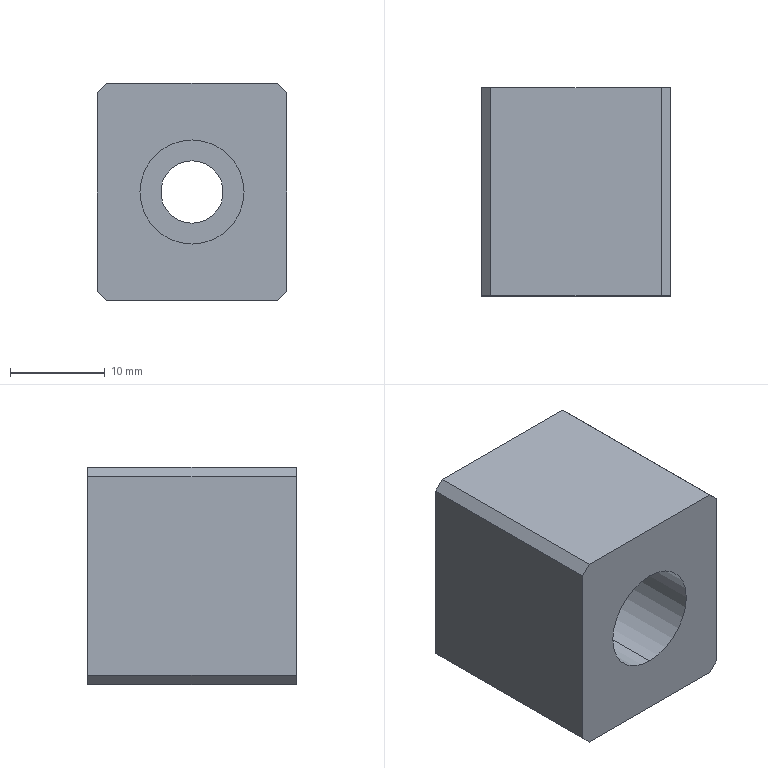Part | SolidWorks | features Chamfer 1, Extrusion 1, HoleWzd 1 | 1 solid | 15 faces | box 20 x 22 x 23 mm | volume 8411 mm3 | plane 11 | cylinder 4 | commonest cylinder face diameters 6.6 x2 11 x2
STEP:
#1=CARTESIAN_POINT('',(0.,15.,5.5));
#2=VERTEX_POINT('',#1);
#3=CARTESIAN_POINT('',(0.,15.,-5.5));
#4=VERTEX_POINT('',#3);
#5=CARTESIAN_POINT('',(0.,15.,0.));
#6=DIRECTION('',(0.,-1.,0.));
#7=DIRECTION('',(0.,0.,-1.));
#8=AXIS2_PLACEMENT_3D('',#5,#6,#7);
#9=CIRCLE('',#8,5.5);
#10=EDGE_CURVE('',#2,#4,#9,.T.);
#11=ORIENTED_EDGE('',*,*,#10,.F.);
#12=CARTESIAN_POINT('',(0.,0.,5.5));
#13=VERTEX_POINT('',#12);
#14=CARTESIAN_POINT('',(0.,0.,5.5));
#15=DIRECTION('',(0.,-1.,0.));
#16=VECTOR('',#15,1000.);
#17=LINE('',#14,#16);
#18=EDGE_CURVE('',#2,#13,#17,.T.);
#19=ORIENTED_EDGE('',*,*,#18,.T.);
#20=CARTESIAN_POINT('',(0.,0.,-5.5));
#21=VERTEX_POINT('',#20);
#22=CARTESIAN_POINT('',(0.,0.,0.));
#23=DIRECTION('',(0.,-1.,0.));
#24=DIRECTION('',(0.,0.,-1.));
#25=AXIS2_PLACEMENT_3D('',#22,#23,#24);
#26=CIRCLE('',#25,5.5);
#27=EDGE_CURVE('',#13,#21,#26,.T.);
#28=ORIENTED_EDGE('',*,*,#27,.T.);
#29=CARTESIAN_POINT('',(0.,0.,-5.5));
#30=DIRECTION('',(0.,-1.,0.));
#31=VECTOR('',#30,1000.);
#32=LINE('',#29,#31);
#33=EDGE_CURVE('',#4,#21,#32,.T.);
#34=ORIENTED_EDGE('',*,*,#33,.F.);
#35=EDGE_LOOP('',(#11,#19,#28,#34));
#36=FACE_OUTER_BOUND('',#35,.T.);
#37=CARTESIAN_POINT('',(0.,0.,0.));
#38=DIRECTION('',(0.,-1.,0.));
#39=DIRECTION('',(0.,0.,-1.));
#40=AXIS2_PLACEMENT_3D('',#37,#38,#39);
#41=CYLINDRICAL_SURFACE('',#40,5.5);
#42=ADVANCED_FACE('',(#36),#41,.F.);
#43=CARTESIAN_POINT('',(0.,22.,-3.3));
#44=VERTEX_POINT('',#43);
#45=CARTESIAN_POINT('',(0.,22.,3.3));
#46=VERTEX_POINT('',#45);
#47=CARTESIAN_POINT('',(0.,22.,0.));
#48=DIRECTION('',(0.,1.,0.));
#49=DIRECTION('',(0.,0.,1.));
#50=AXIS2_PLACEMENT_3D('',#47,#48,#49);
#51=CIRCLE('',#50,3.3);
#52=EDGE_CURVE('',#44,#46,#51,.T.);
#53=ORIENTED_EDGE('',*,*,#52,.T.);
#54=CARTESIAN_POINT('',(0.,15.,3.3));
#55=VERTEX_POINT('',#54);
#56=CARTESIAN_POINT('',(0.,0.,3.3));
#57=DIRECTION('',(0.,-1.,0.));
#58=VECTOR('',#57,1000.);
#59=LINE('',#56,#58);
#60=EDGE_CURVE('',#46,#55,#59,.T.);
#61=ORIENTED_EDGE('',*,*,#60,.T.);
#62=CARTESIAN_POINT('',(0.,15.,-3.3));
#63=VERTEX_POINT('',#62);
#64=CARTESIAN_POINT('',(0.,15.,0.));
#65=DIRECTION('',(0.,-1.,0.));
#66=DIRECTION('',(0.,0.,-1.));
#67=AXIS2_PLACEMENT_3D('',#64,#65,#66);
#68=CIRCLE('',#67,3.3);
#69=EDGE_CURVE('',#55,#63,#68,.T.);
#70=ORIENTED_EDGE('',*,*,#69,.T.);
#71=CARTESIAN_POINT('',(0.,0.,-3.3));
#72=DIRECTION('',(0.,-1.,0.));
#73=VECTOR('',#72,1000.);
#74=LINE('',#71,#73);
#75=EDGE_CURVE('',#44,#63,#74,.T.);
#76=ORIENTED_EDGE('',*,*,#75,.F.);
#77=EDGE_LOOP('',(#53,#61,#70,#76));
#78=FACE_OUTER_BOUND('',#77,.T.);
#79=CARTESIAN_POINT('',(0.,0.,0.));
#80=DIRECTION('',(0.,-1.,0.));
#81=DIRECTION('',(0.,0.,-1.));
#82=AXIS2_PLACEMENT_3D('',#79,#80,#81);
#83=CYLINDRICAL_SURFACE('',#82,3.3);
#84=ADVANCED_FACE('',(#78),#83,.F.);
#85=CARTESIAN_POINT('',(10.,22.,10.5));
#86=VERTEX_POINT('',#85);
#87=CARTESIAN_POINT('',(10.,22.,-10.5));
#88=VERTEX_POINT('',#87);
#89=CARTESIAN_POINT('',(10.,22.,-11.5));
#90=DIRECTION('',(0.,0.,-1.));
#91=VECTOR('',#90,1000.);
#92=LINE('',#89,#91);
#93=EDGE_CURVE('',#86,#88,#92,.T.);
#94=ORIENTED_EDGE('',*,*,#93,.F.);
#95=CARTESIAN_POINT('',(10.,0.,10.5));
#96=VERTEX_POINT('',#95);
#97=CARTESIAN_POINT('',(10.,22.,10.5));
#98=DIRECTION('',(0.,-1.,0.));
#99=VECTOR('',#98,1000.);
#100=LINE('',#97,#99);
#101=EDGE_CURVE('',#86,#96,#100,.T.);
#102=ORIENTED_EDGE('',*,*,#101,.T.);
#103=CARTESIAN_POINT('',(10.,0.,-10.5));
#104=VERTEX_POINT('',#103);
#105=CARTESIAN_POINT('',(10.,0.,-11.5));
#106=DIRECTION('',(0.,0.,-1.));
#107=VECTOR('',#106,1000.);
#108=LINE('',#105,#107);
#109=EDGE_CURVE('',#96,#104,#108,.T.);
#110=ORIENTED_EDGE('',*,*,#109,.T.);
#111=CARTESIAN_POINT('',(10.,22.,-10.5));
#112=DIRECTION('',(0.,1.,0.));
#113=VECTOR('',#112,1000.);
#114=LINE('',#111,#113);
#115=EDGE_CURVE('',#104,#88,#114,.T.);
#116=ORIENTED_EDGE('',*,*,#115,.T.);
#117=EDGE_LOOP('',(#94,#102,#110,#116));
#118=FACE_OUTER_BOUND('',#117,.T.);
#119=CARTESIAN_POINT('',(10.,22.,-11.5));
#120=DIRECTION('',(-1.,0.,0.));
#121=DIRECTION('',(0.,0.,1.));
#122=AXIS2_PLACEMENT_3D('',#119,#120,#121);
#123=PLANE('',#122);
#124=ADVANCED_FACE('',(#118),#123,.F.);
#125=CARTESIAN_POINT('',(9.,22.,-11.5));
#126=VERTEX_POINT('',#125);
#127=CARTESIAN_POINT('',(-9.,22.,-11.5));
#128=VERTEX_POINT('',#127);
#129=CARTESIAN_POINT('',(-10.,22.,-11.5));
#130=DIRECTION('',(-1.,0.,0.));
#131=VECTOR('',#130,1000.);
#132=LINE('',#129,#131);
#133=EDGE_CURVE('',#126,#128,#132,.T.);
#134=ORIENTED_EDGE('',*,*,#133,.F.);
#135=CARTESIAN_POINT('',(9.,0.,-11.5));
#136=VERTEX_POINT('',#135);
#137=CARTESIAN_POINT('',(9.,22.,-11.5));
#138=DIRECTION('',(0.,-1.,0.));
#139=VECTOR('',#138,1000.);
#140=LINE('',#137,#139);
#141=EDGE_CURVE('',#126,#136,#140,.T.);
#142=ORIENTED_EDGE('',*,*,#141,.T.);
#143=CARTESIAN_POINT('',(-9.,0.,-11.5));
#144=VERTEX_POINT('',#143);
#145=CARTESIAN_POINT('',(-10.,0.,-11.5));
#146=DIRECTION('',(-1.,0.,0.));
#147=VECTOR('',#146,1000.);
#148=LINE('',#145,#147);
#149=EDGE_CURVE('',#136,#144,#148,.T.);
#150=ORIENTED_EDGE('',*,*,#149,.T.);
#151=CARTESIAN_POINT('',(-9.,22.,-11.5));
#152=DIRECTION('',(0.,1.,0.));
#153=VECTOR('',#152,1000.);
#154=LINE('',#151,#153);
#155=EDGE_CURVE('',#144,#128,#154,.T.);
#156=ORIENTED_EDGE('',*,*,#155,.T.);
#157=EDGE_LOOP('',(#134,#142,#150,#156));
#158=FACE_OUTER_BOUND('',#157,.T.);
#159=CARTESIAN_POINT('',(-10.,22.,-11.5));
#160=DIRECTION('',(0.,0.,1.));
#161=DIRECTION('',(1.,0.,0.));
#162=AXIS2_PLACEMENT_3D('',#159,#160,#161);
#163=PLANE('',#162);
#164=ADVANCED_FACE('',(#158),#163,.F.);
#165=CARTESIAN_POINT('',(-10.,22.,-10.5));
#166=VERTEX_POINT('',#165);
#167=CARTESIAN_POINT('',(-10.,22.,10.5));
#168=VERTEX_POINT('',#167);
#169=CARTESIAN_POINT('',(-10.,22.,-11.5));
#170=DIRECTION('',(0.,0.,1.));
#171=VECTOR('',#170,1000.);
#172=LINE('',#169,#171);
#173=EDGE_CURVE('',#166,#168,#172,.T.);
#174=ORIENTED_EDGE('',*,*,#173,.F.);
#175=CARTESIAN_POINT('',(-10.,0.,-10.5));
#176=VERTEX_POINT('',#175);
#177=CARTESIAN_POINT('',(-10.,22.,-10.5));
#178=DIRECTION('',(0.,-1.,0.));
#179=VECTOR('',#178,1000.);
#180=LINE('',#177,#179);
#181=EDGE_CURVE('',#166,#176,#180,.T.);
#182=ORIENTED_EDGE('',*,*,#181,.T.);
#183=CARTESIAN_POINT('',(-10.,0.,10.5));
#184=VERTEX_POINT('',#183);
#185=CARTESIAN_POINT('',(-10.,0.,-11.5));
#186=DIRECTION('',(0.,0.,1.));
#187=VECTOR('',#186,1000.);
#188=LINE('',#185,#187);
#189=EDGE_CURVE('',#176,#184,#188,.T.);
#190=ORIENTED_EDGE('',*,*,#189,.T.);
#191=CARTESIAN_POINT('',(-10.,22.,10.5));
#192=DIRECTION('',(0.,1.,0.));
#193=VECTOR('',#192,1000.);
#194=LINE('',#191,#193);
#195=EDGE_CURVE('',#184,#168,#194,.T.);
#196=ORIENTED_EDGE('',*,*,#195,.T.);
#197=EDGE_LOOP('',(#174,#182,#190,#196));
#198=FACE_OUTER_BOUND('',#197,.T.);
#199=CARTESIAN_POINT('',(-10.,22.,-11.5));
#200=DIRECTION('',(1.,0.,0.));
#201=DIRECTION('',(0.,0.,-1.));
#202=AXIS2_PLACEMENT_3D('',#199,#200,#201);
#203=PLANE('',#202);
#204=ADVANCED_FACE('',(#198),#203,.F.);
#205=CARTESIAN_POINT('',(-9.,0.,11.5));
#206=VERTEX_POINT('',#205);
#207=CARTESIAN_POINT('',(9.,0.,11.5));
#208=VERTEX_POINT('',#207);
#209=CARTESIAN_POINT('',(-10.,0.,11.5));
#210=DIRECTION('',(1.,0.,0.));
#211=VECTOR('',#210,1000.);
#212=LINE('',#209,#211);
#213=EDGE_CURVE('',#206,#208,#212,.T.);
#214=ORIENTED_EDGE('',*,*,#213,.T.);
#215=CARTESIAN_POINT('',(9.,22.,11.5));
#216=VERTEX_POINT('',#215);
#217=CARTESIAN_POINT('',(9.,22.,11.5));
#218=DIRECTION('',(0.,1.,0.));
#219=VECTOR('',#218,1000.);
#220=LINE('',#217,#219);
#221=EDGE_CURVE('',#208,#216,#220,.T.);
#222=ORIENTED_EDGE('',*,*,#221,.T.);
#223=CARTESIAN_POINT('',(-9.,22.,11.5));
#224=VERTEX_POINT('',#223);
#225=CARTESIAN_POINT('',(-10.,22.,11.5));
#226=DIRECTION('',(1.,0.,0.));
#227=VECTOR('',#226,1000.);
#228=LINE('',#225,#227);
#229=EDGE_CURVE('',#224,#216,#228,.T.);
#230=ORIENTED_EDGE('',*,*,#229,.F.);
#231=CARTESIAN_POINT('',(-9.,22.,11.5));
#232=DIRECTION('',(0.,-1.,0.));
#233=VECTOR('',#232,1000.);
#234=LINE('',#231,#233);
#235=EDGE_CURVE('',#224,#206,#234,.T.);
#236=ORIENTED_EDGE('',*,*,#235,.T.);
#237=EDGE_LOOP('',(#214,#222,#230,#236));
#238=FACE_OUTER_BOUND('',#237,.T.);
#239=CARTESIAN_POINT('',(-10.,22.,11.5));
#240=DIRECTION('',(0.,0.,-1.));
#241=DIRECTION('',(-1.,0.,0.));
#242=AXIS2_PLACEMENT_3D('',#239,#240,#241);
#243=PLANE('',#242);
#244=ADVANCED_FACE('',(#238),#243,.F.);
#245=ORIENTED_EDGE('',*,*,#52,.F.);
#246=CARTESIAN_POINT('',(0.,22.,0.));
#247=DIRECTION('',(0.,1.,0.));
#248=DIRECTION('',(0.,0.,1.));
#249=AXIS2_PLACEMENT_3D('',#246,#247,#248);
#250=CIRCLE('',#249,3.3);
#251=EDGE_CURVE('',#46,#44,#250,.T.);
#252=ORIENTED_EDGE('',*,*,#251,.F.);
#253=EDGE_LOOP('',(#245,#252));
#254=FACE_BOUND('',#253,.T.);
#255=ORIENTED_EDGE('',*,*,#229,.T.);
#256=CARTESIAN_POINT('',(10.25,22.,10.25));
#257=DIRECTION('',(0.7071,0.,-0.7071));
#258=VECTOR('',#257,1000.);
#259=LINE('',#256,#258);
#260=EDGE_CURVE('',#216,#86,#259,.T.);
#261=ORIENTED_EDGE('',*,*,#260,.T.);
#262=ORIENTED_EDGE('',*,*,#93,.T.);
#263=CARTESIAN_POINT('',(10.25,22.,-10.25));
#264=DIRECTION('',(-0.7071,0.,-0.7071));
#265=VECTOR('',#264,1000.);
#266=LINE('',#263,#265);
#267=EDGE_CURVE('',#88,#126,#266,.T.);
#268=ORIENTED_EDGE('',*,*,#267,.T.);
#269=ORIENTED_EDGE('',*,*,#133,.T.);
#270=CARTESIAN_POINT('',(-10.25,22.,-10.25));
#271=DIRECTION('',(-0.7071,0.,0.7071));
#272=VECTOR('',#271,1000.);
#273=LINE('',#270,#272);
#274=EDGE_CURVE('',#128,#166,#273,.T.);
#275=ORIENTED_EDGE('',*,*,#274,.T.);
#276=ORIENTED_EDGE('',*,*,#173,.T.);
#277=CARTESIAN_POINT('',(-10.25,22.,10.25));
#278=DIRECTION('',(0.7071,0.,0.7071));
#279=VECTOR('',#278,1000.);
#280=LINE('',#277,#279);
#281=EDGE_CURVE('',#168,#224,#280,.T.);
#282=ORIENTED_EDGE('',*,*,#281,.T.);
#283=EDGE_LOOP('',(#255,#261,#262,#268,#269,#275,#276,#282));
#284=FACE_OUTER_BOUND('',#283,.T.);
#285=CARTESIAN_POINT('',(0.,22.,0.));
#286=DIRECTION('',(0.,1.,0.));
#287=DIRECTION('',(0.,0.,1.));
#288=AXIS2_PLACEMENT_3D('',#285,#286,#287);
#289=PLANE('',#288);
#290=ADVANCED_FACE('',(#254,#284),#289,.T.);
#291=CARTESIAN_POINT('',(0.,0.,0.));
#292=DIRECTION('',(0.,-1.,0.));
#293=DIRECTION('',(0.,0.,-1.));
#294=AXIS2_PLACEMENT_3D('',#291,#292,#293);
#295=CIRCLE('',#294,5.5);
#296=EDGE_CURVE('',#21,#13,#295,.T.);
#297=ORIENTED_EDGE('',*,*,#296,.F.);
#298=ORIENTED_EDGE('',*,*,#27,.F.);
#299=EDGE_LOOP('',(#297,#298));
#300=FACE_BOUND('',#299,.T.);
#301=ORIENTED_EDGE('',*,*,#109,.F.);
#302=CARTESIAN_POINT('',(10.,0.,10.5));
#303=DIRECTION('',(-0.7071,0.,0.7071));
#304=VECTOR('',#303,1000.);
#305=LINE('',#302,#304);
#306=EDGE_CURVE('',#96,#208,#305,.T.);
#307=ORIENTED_EDGE('',*,*,#306,.T.);
#308=ORIENTED_EDGE('',*,*,#213,.F.);
#309=CARTESIAN_POINT('',(-9.,0.,11.5));
#310=DIRECTION('',(-0.7071,0.,-0.7071));
#311=VECTOR('',#310,1000.);
#312=LINE('',#309,#311);
#313=EDGE_CURVE('',#206,#184,#312,.T.);
#314=ORIENTED_EDGE('',*,*,#313,.T.);
#315=ORIENTED_EDGE('',*,*,#189,.F.);
#316=CARTESIAN_POINT('',(-10.,0.,-10.5));
#317=DIRECTION('',(0.7071,0.,-0.7071));
#318=VECTOR('',#317,1000.);
#319=LINE('',#316,#318);
#320=EDGE_CURVE('',#176,#144,#319,.T.);
#321=ORIENTED_EDGE('',*,*,#320,.T.);
#322=ORIENTED_EDGE('',*,*,#149,.F.);
#323=CARTESIAN_POINT('',(9.,0.,-11.5));
#324=DIRECTION('',(0.7071,0.,0.7071));
#325=VECTOR('',#324,1000.);
#326=LINE('',#323,#325);
#327=EDGE_CURVE('',#136,#104,#326,.T.);
#328=ORIENTED_EDGE('',*,*,#327,.T.);
#329=EDGE_LOOP('',(#301,#307,#308,#314,#315,#321,#322,#328));
#330=FACE_OUTER_BOUND('',#329,.T.);
#331=CARTESIAN_POINT('',(0.,0.,0.));
#332=DIRECTION('',(0.,1.,0.));
#333=DIRECTION('',(0.,0.,1.));
#334=AXIS2_PLACEMENT_3D('',#331,#332,#333);
#335=PLANE('',#334);
#336=ADVANCED_FACE('',(#300,#330),#335,.F.);
#337=ORIENTED_EDGE('',*,*,#60,.F.);
#338=ORIENTED_EDGE('',*,*,#251,.T.);
#339=ORIENTED_EDGE('',*,*,#75,.T.);
#340=CARTESIAN_POINT('',(0.,15.,0.));
#341=DIRECTION('',(0.,-1.,0.));
#342=DIRECTION('',(0.,0.,-1.));
#343=AXIS2_PLACEMENT_3D('',#340,#341,#342);
#344=CIRCLE('',#343,3.3);
#345=EDGE_CURVE('',#63,#55,#344,.T.);
#346=ORIENTED_EDGE('',*,*,#345,.T.);
#347=EDGE_LOOP('',(#337,#338,#339,#346));
#348=FACE_OUTER_BOUND('',#347,.T.);
#349=CARTESIAN_POINT('',(0.,0.,0.));
#350=DIRECTION('',(0.,-1.,0.));
#351=DIRECTION('',(0.,0.,-1.));
#352=AXIS2_PLACEMENT_3D('',#349,#350,#351);
#353=CYLINDRICAL_SURFACE('',#352,3.3);
#354=ADVANCED_FACE('',(#348),#353,.F.);
#355=ORIENTED_EDGE('',*,*,#345,.F.);
#356=ORIENTED_EDGE('',*,*,#69,.F.);
#357=EDGE_LOOP('',(#355,#356));
#358=FACE_BOUND('',#357,.T.);
#359=CARTESIAN_POINT('',(0.,15.,0.));
#360=DIRECTION('',(0.,-1.,0.));
#361=DIRECTION('',(0.,0.,-1.));
#362=AXIS2_PLACEMENT_3D('',#359,#360,#361);
#363=CIRCLE('',#362,5.5);
#364=EDGE_CURVE('',#4,#2,#363,.T.);
#365=ORIENTED_EDGE('',*,*,#364,.T.);
#366=ORIENTED_EDGE('',*,*,#10,.T.);
#367=EDGE_LOOP('',(#365,#366));
#368=FACE_OUTER_BOUND('',#367,.T.);
#369=CARTESIAN_POINT('',(3.3,15.,0.));
#370=DIRECTION('',(0.,1.,0.));
#371=DIRECTION('',(0.,0.,1.));
#372=AXIS2_PLACEMENT_3D('',#369,#370,#371);
#373=PLANE('',#372);
#374=ADVANCED_FACE('',(#358,#368),#373,.F.);
#375=ORIENTED_EDGE('',*,*,#18,.F.);
#376=ORIENTED_EDGE('',*,*,#364,.F.);
#377=ORIENTED_EDGE('',*,*,#33,.T.);
#378=ORIENTED_EDGE('',*,*,#296,.T.);
#379=EDGE_LOOP('',(#375,#376,#377,#378));
#380=FACE_OUTER_BOUND('',#379,.T.);
#381=CARTESIAN_POINT('',(0.,0.,0.));
#382=DIRECTION('',(0.,-1.,0.));
#383=DIRECTION('',(0.,0.,-1.));
#384=AXIS2_PLACEMENT_3D('',#381,#382,#383);
#385=CYLINDRICAL_SURFACE('',#384,5.5);
#386=ADVANCED_FACE('',(#380),#385,.F.);
#387=ORIENTED_EDGE('',*,*,#260,.F.);
#388=ORIENTED_EDGE('',*,*,#221,.F.);
#389=ORIENTED_EDGE('',*,*,#306,.F.);
#390=ORIENTED_EDGE('',*,*,#101,.F.);
#391=EDGE_LOOP('',(#387,#388,#389,#390));
#392=FACE_OUTER_BOUND('',#391,.T.);
#393=CARTESIAN_POINT('',(10.,22.,10.5));
#394=DIRECTION('',(-0.7071,0.,-0.7071));
#395=DIRECTION('',(0.,-1.,0.));
#396=AXIS2_PLACEMENT_3D('',#393,#394,#395);
#397=PLANE('',#396);
#398=ADVANCED_FACE('',(#392),#397,.F.);
#399=ORIENTED_EDGE('',*,*,#267,.F.);
#400=ORIENTED_EDGE('',*,*,#115,.F.);
#401=ORIENTED_EDGE('',*,*,#327,.F.);
#402=ORIENTED_EDGE('',*,*,#141,.F.);
#403=EDGE_LOOP('',(#399,#400,#401,#402));
#404=FACE_OUTER_BOUND('',#403,.T.);
#405=CARTESIAN_POINT('',(9.,22.,-11.5));
#406=DIRECTION('',(-0.7071,0.,0.7071));
#407=DIRECTION('',(0.,-1.,0.));
#408=AXIS2_PLACEMENT_3D('',#405,#406,#407);
#409=PLANE('',#408);
#410=ADVANCED_FACE('',(#404),#409,.F.);
#411=ORIENTED_EDGE('',*,*,#274,.F.);
#412=ORIENTED_EDGE('',*,*,#155,.F.);
#413=ORIENTED_EDGE('',*,*,#320,.F.);
#414=ORIENTED_EDGE('',*,*,#181,.F.);
#415=EDGE_LOOP('',(#411,#412,#413,#414));
#416=FACE_OUTER_BOUND('',#415,.T.);
#417=CARTESIAN_POINT('',(-10.,22.,-10.5));
#418=DIRECTION('',(0.7071,0.,0.7071));
#419=DIRECTION('',(0.,-1.,0.));
#420=AXIS2_PLACEMENT_3D('',#417,#418,#419);
#421=PLANE('',#420);
#422=ADVANCED_FACE('',(#416),#421,.F.);
#423=ORIENTED_EDGE('',*,*,#281,.F.);
#424=ORIENTED_EDGE('',*,*,#195,.F.);
#425=ORIENTED_EDGE('',*,*,#313,.F.);
#426=ORIENTED_EDGE('',*,*,#235,.F.);
#427=EDGE_LOOP('',(#423,#424,#425,#426));
#428=FACE_OUTER_BOUND('',#427,.T.);
#429=CARTESIAN_POINT('',(-9.,22.,11.5));
#430=DIRECTION('',(0.7071,0.,-0.7071));
#431=DIRECTION('',(0.,-1.,0.));
#432=AXIS2_PLACEMENT_3D('',#429,#430,#431);
#433=PLANE('',#432);
#434=ADVANCED_FACE('',(#428),#433,.F.);
#435=CLOSED_SHELL('',(#42,#84,#124,#164,#204,#244,#290,#336,#354,#374,#386,#398,#410,#422,#434));
#436=MANIFOLD_SOLID_BREP('',#435);
#437=CARTESIAN_POINT('',(0.,0.,0.));
#438=DIRECTION('',(0.,0.,1.));
#439=DIRECTION('',(1.,0.,0.));
#440=AXIS2_PLACEMENT_3D('',#437,#438,#439);
#441=(LENGTH_UNIT()NAMED_UNIT(*)SI_UNIT(.MILLI.,.METRE.));
#442=UNCERTAINTY_MEASURE_WITH_UNIT(LENGTH_MEASURE(0.00001),#441,'','');
#443=(NAMED_UNIT(*)PLANE_ANGLE_UNIT()SI_UNIT($,.RADIAN.));
#444=(NAMED_UNIT(*)SI_UNIT($,.STERADIAN.)SOLID_ANGLE_UNIT());
#445=(GEOMETRIC_REPRESENTATION_CONTEXT(3)GLOBAL_UNCERTAINTY_ASSIGNED_CONTEXT((#442))GLOBAL_UNIT_ASSIGNED_CONTEXT((#441,#443,#444))REPRESENTATION_CONTEXT('',''));
#446=ADVANCED_BREP_SHAPE_REPRESENTATION('',(#436,#440),#445);